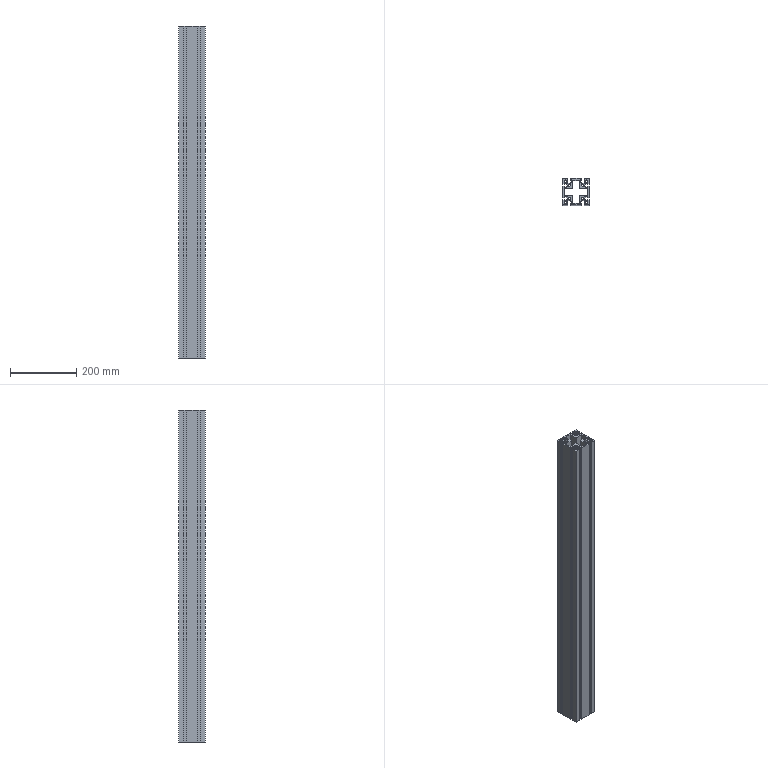Part | NX | features BREP 1 | 1 solid | 130 faces | box 80 x 80 x 1000 mm | volume 2460666 mm3 | plane 114 | cylinder 16 | commonest cylinder face diameters 6.8 x16